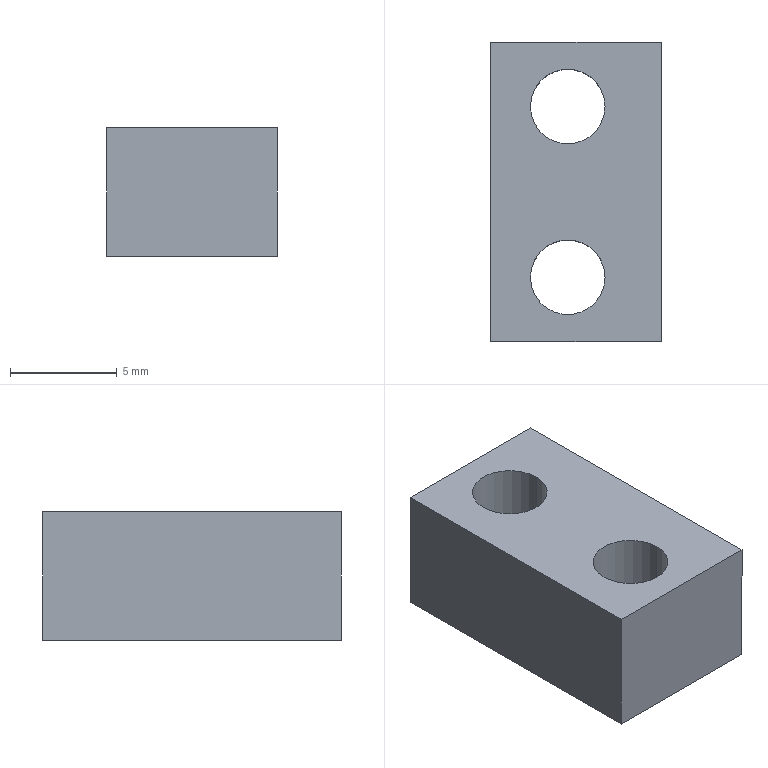Part | SolidWorks | features BaseBody 1 | 1 solid | 10 faces | box 8 x 14 x 6 mm | volume 556.546 mm3 | plane 6 | cylinder 4 | commonest cylinder face diameters 3.5 x4
STEP:
#1=CARTESIAN_POINT('',(-8.25,3.,0.));
#2=VERTEX_POINT('',#1);
#3=CARTESIAN_POINT('',(-11.75,3.,0.));
#4=VERTEX_POINT('',#3);
#5=CARTESIAN_POINT('',(-10.,3.,0.));
#6=DIRECTION('',(0.,0.,-1.));
#7=DIRECTION('',(1.,0.,0.));
#8=AXIS2_PLACEMENT_3D('',#5,#6,#7);
#9=CIRCLE('',#8,1.75);
#10=EDGE_CURVE('',#2,#4,#9,.T.);
#11=ORIENTED_EDGE('',*,*,#10,.T.);
#12=CARTESIAN_POINT('',(-11.75,3.,6.));
#13=VERTEX_POINT('',#12);
#14=CARTESIAN_POINT('',(-11.75,3.,-11.205));
#15=DIRECTION('',(0.,0.,1.));
#16=VECTOR('',#15,1000.);
#17=LINE('',#14,#16);
#18=EDGE_CURVE('',#4,#13,#17,.T.);
#19=ORIENTED_EDGE('',*,*,#18,.T.);
#20=CARTESIAN_POINT('',(-8.25,3.,6.));
#21=VERTEX_POINT('',#20);
#22=CARTESIAN_POINT('',(-10.,3.,6.));
#23=DIRECTION('',(0.,0.,-1.));
#24=DIRECTION('',(1.,0.,0.));
#25=AXIS2_PLACEMENT_3D('',#22,#23,#24);
#26=CIRCLE('',#25,1.75);
#27=EDGE_CURVE('',#21,#13,#26,.T.);
#28=ORIENTED_EDGE('',*,*,#27,.F.);
#29=CARTESIAN_POINT('',(-8.25,3.,-11.205));
#30=DIRECTION('',(0.,0.,1.));
#31=VECTOR('',#30,1000.);
#32=LINE('',#29,#31);
#33=EDGE_CURVE('',#2,#21,#32,.T.);
#34=ORIENTED_EDGE('',*,*,#33,.F.);
#35=EDGE_LOOP('',(#11,#19,#28,#34));
#36=FACE_OUTER_BOUND('',#35,.T.);
#37=CARTESIAN_POINT('',(-10.,3.,-11.205));
#38=DIRECTION('',(0.,0.,1.));
#39=DIRECTION('',(1.,0.,0.));
#40=AXIS2_PLACEMENT_3D('',#37,#38,#39);
#41=CYLINDRICAL_SURFACE('',#40,1.75);
#42=ADVANCED_FACE('',(#36),#41,.F.);
#43=CARTESIAN_POINT('',(-8.25,11.,0.));
#44=VERTEX_POINT('',#43);
#45=CARTESIAN_POINT('',(-11.75,11.,0.));
#46=VERTEX_POINT('',#45);
#47=CARTESIAN_POINT('',(-10.,11.,0.));
#48=DIRECTION('',(0.,0.,-1.));
#49=DIRECTION('',(1.,0.,0.));
#50=AXIS2_PLACEMENT_3D('',#47,#48,#49);
#51=CIRCLE('',#50,1.75);
#52=EDGE_CURVE('',#44,#46,#51,.T.);
#53=ORIENTED_EDGE('',*,*,#52,.T.);
#54=CARTESIAN_POINT('',(-11.75,11.,6.));
#55=VERTEX_POINT('',#54);
#56=CARTESIAN_POINT('',(-11.75,11.,-11.205));
#57=DIRECTION('',(0.,0.,1.));
#58=VECTOR('',#57,1000.);
#59=LINE('',#56,#58);
#60=EDGE_CURVE('',#46,#55,#59,.T.);
#61=ORIENTED_EDGE('',*,*,#60,.T.);
#62=CARTESIAN_POINT('',(-8.25,11.,6.));
#63=VERTEX_POINT('',#62);
#64=CARTESIAN_POINT('',(-10.,11.,6.));
#65=DIRECTION('',(0.,0.,-1.));
#66=DIRECTION('',(1.,0.,0.));
#67=AXIS2_PLACEMENT_3D('',#64,#65,#66);
#68=CIRCLE('',#67,1.75);
#69=EDGE_CURVE('',#63,#55,#68,.T.);
#70=ORIENTED_EDGE('',*,*,#69,.F.);
#71=CARTESIAN_POINT('',(-8.25,11.,-11.205));
#72=DIRECTION('',(0.,0.,1.));
#73=VECTOR('',#72,1000.);
#74=LINE('',#71,#73);
#75=EDGE_CURVE('',#44,#63,#74,.T.);
#76=ORIENTED_EDGE('',*,*,#75,.F.);
#77=EDGE_LOOP('',(#53,#61,#70,#76));
#78=FACE_OUTER_BOUND('',#77,.T.);
#79=CARTESIAN_POINT('',(-10.,11.,-11.205));
#80=DIRECTION('',(0.,0.,1.));
#81=DIRECTION('',(1.,0.,0.));
#82=AXIS2_PLACEMENT_3D('',#79,#80,#81);
#83=CYLINDRICAL_SURFACE('',#82,1.75);
#84=ADVANCED_FACE('',(#78),#83,.F.);
#85=ORIENTED_EDGE('',*,*,#10,.F.);
#86=CARTESIAN_POINT('',(-10.,3.,0.));
#87=DIRECTION('',(0.,0.,-1.));
#88=DIRECTION('',(1.,0.,0.));
#89=AXIS2_PLACEMENT_3D('',#86,#87,#88);
#90=CIRCLE('',#89,1.75);
#91=EDGE_CURVE('',#4,#2,#90,.T.);
#92=ORIENTED_EDGE('',*,*,#91,.F.);
#93=EDGE_LOOP('',(#85,#92));
#94=FACE_BOUND('',#93,.T.);
#95=ORIENTED_EDGE('',*,*,#52,.F.);
#96=CARTESIAN_POINT('',(-10.,11.,0.));
#97=DIRECTION('',(0.,0.,-1.));
#98=DIRECTION('',(1.,0.,0.));
#99=AXIS2_PLACEMENT_3D('',#96,#97,#98);
#100=CIRCLE('',#99,1.75);
#101=EDGE_CURVE('',#46,#44,#100,.T.);
#102=ORIENTED_EDGE('',*,*,#101,.F.);
#103=EDGE_LOOP('',(#95,#102));
#104=FACE_BOUND('',#103,.T.);
#105=CARTESIAN_POINT('',(-5.612,0.,0.));
#106=VERTEX_POINT('',#105);
#107=CARTESIAN_POINT('',(-5.612,14.,0.));
#108=VERTEX_POINT('',#107);
#109=CARTESIAN_POINT('',(-5.612,7.,0.));
#110=DIRECTION('',(0.,1.,0.));
#111=VECTOR('',#110,1000.);
#112=LINE('',#109,#111);
#113=EDGE_CURVE('',#106,#108,#112,.T.);
#114=ORIENTED_EDGE('',*,*,#113,.F.);
#115=CARTESIAN_POINT('',(-13.612,0.,0.));
#116=VERTEX_POINT('',#115);
#117=CARTESIAN_POINT('',(-9.612,0.,0.));
#118=DIRECTION('',(1.,0.,0.));
#119=VECTOR('',#118,1000.);
#120=LINE('',#117,#119);
#121=EDGE_CURVE('',#116,#106,#120,.T.);
#122=ORIENTED_EDGE('',*,*,#121,.F.);
#123=CARTESIAN_POINT('',(-13.612,14.,0.));
#124=VERTEX_POINT('',#123);
#125=CARTESIAN_POINT('',(-13.612,7.,0.));
#126=DIRECTION('',(0.,-1.,0.));
#127=VECTOR('',#126,1000.);
#128=LINE('',#125,#127);
#129=EDGE_CURVE('',#124,#116,#128,.T.);
#130=ORIENTED_EDGE('',*,*,#129,.F.);
#131=CARTESIAN_POINT('',(-9.612,14.,0.));
#132=DIRECTION('',(-1.,0.,0.));
#133=VECTOR('',#132,1000.);
#134=LINE('',#131,#133);
#135=EDGE_CURVE('',#108,#124,#134,.T.);
#136=ORIENTED_EDGE('',*,*,#135,.F.);
#137=EDGE_LOOP('',(#114,#122,#130,#136));
#138=FACE_OUTER_BOUND('',#137,.T.);
#139=CARTESIAN_POINT('',(-9.612,7.,0.));
#140=DIRECTION('',(0.,0.,1.));
#141=DIRECTION('',(1.,0.,0.));
#142=AXIS2_PLACEMENT_3D('',#139,#140,#141);
#143=PLANE('',#142);
#144=ADVANCED_FACE('',(#94,#104,#138),#143,.F.);
#145=ORIENTED_EDGE('',*,*,#18,.F.);
#146=ORIENTED_EDGE('',*,*,#91,.T.);
#147=ORIENTED_EDGE('',*,*,#33,.T.);
#148=CARTESIAN_POINT('',(-10.,3.,6.));
#149=DIRECTION('',(0.,0.,-1.));
#150=DIRECTION('',(1.,0.,0.));
#151=AXIS2_PLACEMENT_3D('',#148,#149,#150);
#152=CIRCLE('',#151,1.75);
#153=EDGE_CURVE('',#13,#21,#152,.T.);
#154=ORIENTED_EDGE('',*,*,#153,.F.);
#155=EDGE_LOOP('',(#145,#146,#147,#154));
#156=FACE_OUTER_BOUND('',#155,.T.);
#157=CARTESIAN_POINT('',(-10.,3.,-11.205));
#158=DIRECTION('',(0.,0.,1.));
#159=DIRECTION('',(1.,0.,0.));
#160=AXIS2_PLACEMENT_3D('',#157,#158,#159);
#161=CYLINDRICAL_SURFACE('',#160,1.75);
#162=ADVANCED_FACE('',(#156),#161,.F.);
#163=ORIENTED_EDGE('',*,*,#60,.F.);
#164=ORIENTED_EDGE('',*,*,#101,.T.);
#165=ORIENTED_EDGE('',*,*,#75,.T.);
#166=CARTESIAN_POINT('',(-10.,11.,6.));
#167=DIRECTION('',(0.,0.,-1.));
#168=DIRECTION('',(1.,0.,0.));
#169=AXIS2_PLACEMENT_3D('',#166,#167,#168);
#170=CIRCLE('',#169,1.75);
#171=EDGE_CURVE('',#55,#63,#170,.T.);
#172=ORIENTED_EDGE('',*,*,#171,.F.);
#173=EDGE_LOOP('',(#163,#164,#165,#172));
#174=FACE_OUTER_BOUND('',#173,.T.);
#175=CARTESIAN_POINT('',(-10.,11.,-11.205));
#176=DIRECTION('',(0.,0.,1.));
#177=DIRECTION('',(1.,0.,0.));
#178=AXIS2_PLACEMENT_3D('',#175,#176,#177);
#179=CYLINDRICAL_SURFACE('',#178,1.75);
#180=ADVANCED_FACE('',(#174),#179,.F.);
#181=ORIENTED_EDGE('',*,*,#135,.T.);
#182=CARTESIAN_POINT('',(-13.612,14.,6.));
#183=VERTEX_POINT('',#182);
#184=CARTESIAN_POINT('',(-13.612,14.,0.));
#185=DIRECTION('',(0.,0.,1.));
#186=VECTOR('',#185,1000.);
#187=LINE('',#184,#186);
#188=EDGE_CURVE('',#124,#183,#187,.T.);
#189=ORIENTED_EDGE('',*,*,#188,.T.);
#190=CARTESIAN_POINT('',(-5.612,14.,6.));
#191=VERTEX_POINT('',#190);
#192=CARTESIAN_POINT('',(-13.612,14.,6.));
#193=DIRECTION('',(1.,0.,0.));
#194=VECTOR('',#193,1000.);
#195=LINE('',#192,#194);
#196=EDGE_CURVE('',#183,#191,#195,.T.);
#197=ORIENTED_EDGE('',*,*,#196,.T.);
#198=CARTESIAN_POINT('',(-5.612,14.,0.));
#199=DIRECTION('',(0.,0.,-1.));
#200=VECTOR('',#199,1000.);
#201=LINE('',#198,#200);
#202=EDGE_CURVE('',#191,#108,#201,.T.);
#203=ORIENTED_EDGE('',*,*,#202,.T.);
#204=EDGE_LOOP('',(#181,#189,#197,#203));
#205=FACE_OUTER_BOUND('',#204,.T.);
#206=CARTESIAN_POINT('',(-13.612,14.,0.));
#207=DIRECTION('',(0.,1.,0.));
#208=DIRECTION('',(0.,0.,1.));
#209=AXIS2_PLACEMENT_3D('',#206,#207,#208);
#210=PLANE('',#209);
#211=ADVANCED_FACE('',(#205),#210,.T.);
#212=ORIENTED_EDGE('',*,*,#113,.T.);
#213=ORIENTED_EDGE('',*,*,#202,.F.);
#214=CARTESIAN_POINT('',(-5.612,0.,6.));
#215=VERTEX_POINT('',#214);
#216=CARTESIAN_POINT('',(-5.612,14.,6.));
#217=DIRECTION('',(0.,-1.,0.));
#218=VECTOR('',#217,1000.);
#219=LINE('',#216,#218);
#220=EDGE_CURVE('',#191,#215,#219,.T.);
#221=ORIENTED_EDGE('',*,*,#220,.T.);
#222=CARTESIAN_POINT('',(-5.612,0.,0.));
#223=DIRECTION('',(0.,0.,-1.));
#224=VECTOR('',#223,1000.);
#225=LINE('',#222,#224);
#226=EDGE_CURVE('',#215,#106,#225,.T.);
#227=ORIENTED_EDGE('',*,*,#226,.T.);
#228=EDGE_LOOP('',(#212,#213,#221,#227));
#229=FACE_OUTER_BOUND('',#228,.T.);
#230=CARTESIAN_POINT('',(-5.612,14.,0.));
#231=DIRECTION('',(1.,0.,0.));
#232=DIRECTION('',(0.,0.,-1.));
#233=AXIS2_PLACEMENT_3D('',#230,#231,#232);
#234=PLANE('',#233);
#235=ADVANCED_FACE('',(#229),#234,.T.);
#236=ORIENTED_EDGE('',*,*,#121,.T.);
#237=ORIENTED_EDGE('',*,*,#226,.F.);
#238=CARTESIAN_POINT('',(-13.612,0.,6.));
#239=VERTEX_POINT('',#238);
#240=CARTESIAN_POINT('',(-5.612,0.,6.));
#241=DIRECTION('',(-1.,0.,0.));
#242=VECTOR('',#241,1000.);
#243=LINE('',#240,#242);
#244=EDGE_CURVE('',#215,#239,#243,.T.);
#245=ORIENTED_EDGE('',*,*,#244,.T.);
#246=CARTESIAN_POINT('',(-13.612,0.,0.));
#247=DIRECTION('',(0.,0.,-1.));
#248=VECTOR('',#247,1000.);
#249=LINE('',#246,#248);
#250=EDGE_CURVE('',#239,#116,#249,.T.);
#251=ORIENTED_EDGE('',*,*,#250,.T.);
#252=EDGE_LOOP('',(#236,#237,#245,#251));
#253=FACE_OUTER_BOUND('',#252,.T.);
#254=CARTESIAN_POINT('',(-5.612,0.,0.));
#255=DIRECTION('',(0.,-1.,0.));
#256=DIRECTION('',(0.,0.,-1.));
#257=AXIS2_PLACEMENT_3D('',#254,#255,#256);
#258=PLANE('',#257);
#259=ADVANCED_FACE('',(#253),#258,.T.);
#260=ORIENTED_EDGE('',*,*,#129,.T.);
#261=ORIENTED_EDGE('',*,*,#250,.F.);
#262=CARTESIAN_POINT('',(-13.612,0.,6.));
#263=DIRECTION('',(0.,1.,0.));
#264=VECTOR('',#263,1000.);
#265=LINE('',#262,#264);
#266=EDGE_CURVE('',#239,#183,#265,.T.);
#267=ORIENTED_EDGE('',*,*,#266,.T.);
#268=ORIENTED_EDGE('',*,*,#188,.F.);
#269=EDGE_LOOP('',(#260,#261,#267,#268));
#270=FACE_OUTER_BOUND('',#269,.T.);
#271=CARTESIAN_POINT('',(-13.612,0.,0.));
#272=DIRECTION('',(-1.,0.,0.));
#273=DIRECTION('',(0.,0.,1.));
#274=AXIS2_PLACEMENT_3D('',#271,#272,#273);
#275=PLANE('',#274);
#276=ADVANCED_FACE('',(#270),#275,.T.);
#277=ORIENTED_EDGE('',*,*,#27,.T.);
#278=ORIENTED_EDGE('',*,*,#153,.T.);
#279=EDGE_LOOP('',(#277,#278));
#280=FACE_BOUND('',#279,.T.);
#281=ORIENTED_EDGE('',*,*,#69,.T.);
#282=ORIENTED_EDGE('',*,*,#171,.T.);
#283=EDGE_LOOP('',(#281,#282));
#284=FACE_BOUND('',#283,.T.);
#285=ORIENTED_EDGE('',*,*,#266,.F.);
#286=ORIENTED_EDGE('',*,*,#244,.F.);
#287=ORIENTED_EDGE('',*,*,#220,.F.);
#288=ORIENTED_EDGE('',*,*,#196,.F.);
#289=EDGE_LOOP('',(#285,#286,#287,#288));
#290=FACE_OUTER_BOUND('',#289,.T.);
#291=CARTESIAN_POINT('',(-9.612,7.,6.));
#292=DIRECTION('',(0.,0.,1.));
#293=DIRECTION('',(1.,0.,0.));
#294=AXIS2_PLACEMENT_3D('',#291,#292,#293);
#295=PLANE('',#294);
#296=ADVANCED_FACE('',(#280,#284,#290),#295,.T.);
#297=CLOSED_SHELL('',(#42,#84,#144,#162,#180,#211,#235,#259,#276,#296));
#298=MANIFOLD_SOLID_BREP('',#297);
#299=CARTESIAN_POINT('',(0.,0.,0.));
#300=DIRECTION('',(0.,0.,1.));
#301=DIRECTION('',(1.,0.,0.));
#302=AXIS2_PLACEMENT_3D('',#299,#300,#301);
#303=(LENGTH_UNIT()NAMED_UNIT(*)SI_UNIT(.MILLI.,.METRE.));
#304=UNCERTAINTY_MEASURE_WITH_UNIT(LENGTH_MEASURE(0.00001),#303,'','');
#305=(NAMED_UNIT(*)PLANE_ANGLE_UNIT()SI_UNIT($,.RADIAN.));
#306=(NAMED_UNIT(*)SI_UNIT($,.STERADIAN.)SOLID_ANGLE_UNIT());
#307=(GEOMETRIC_REPRESENTATION_CONTEXT(3)GLOBAL_UNCERTAINTY_ASSIGNED_CONTEXT((#304))GLOBAL_UNIT_ASSIGNED_CONTEXT((#303,#305,#306))REPRESENTATION_CONTEXT('',''));
#308=ADVANCED_BREP_SHAPE_REPRESENTATION('',(#298,#302),#307);